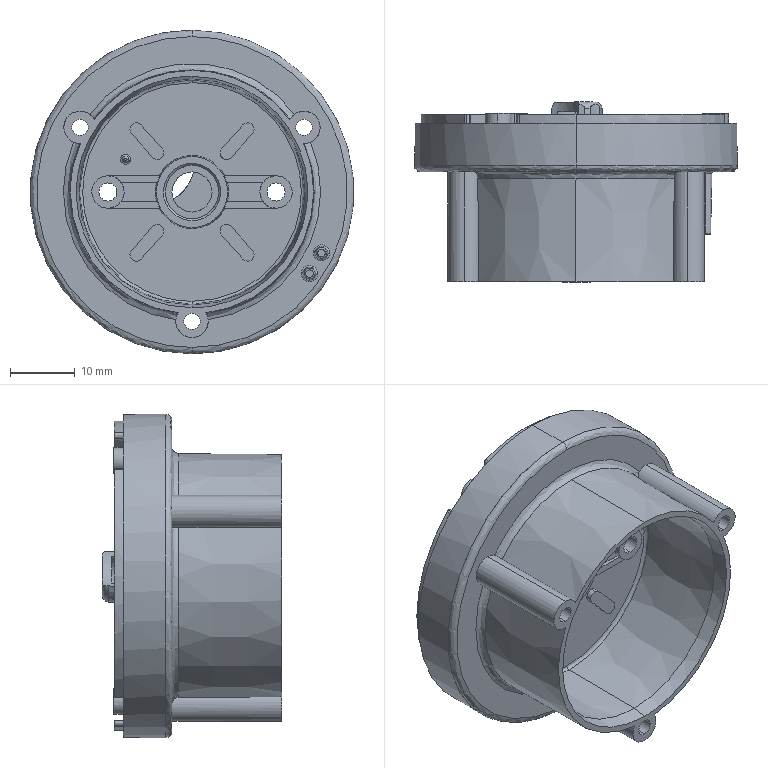Part | SolidWorks | features BaseBody 1 | 1 solid | 245 faces | box 50.06 x 27.8 x 50.06 mm | volume 10061 mm3 | cylinder 114 | plane 64 | cone 42 | spline 23 | torus 2 | commonest cylinder face diameters 2 x20 4 x16 5 x12 1.95 x10 1.087 x8 2.5 x6